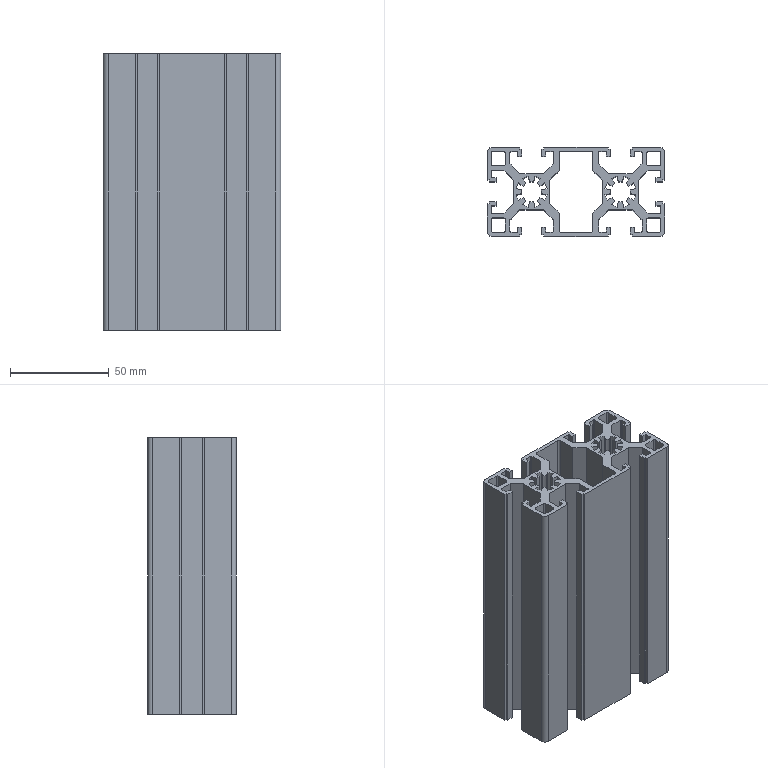Part | STEP file | OB4590-L4 | 1 solid | 256 faces | box 90 x 45 x 140 mm | volume 178928 mm3 | plane 174 | cylinder 82 | commonest cylinder face diameters 1 x24 2 x20 10.2 x18 16 x16 5 x4